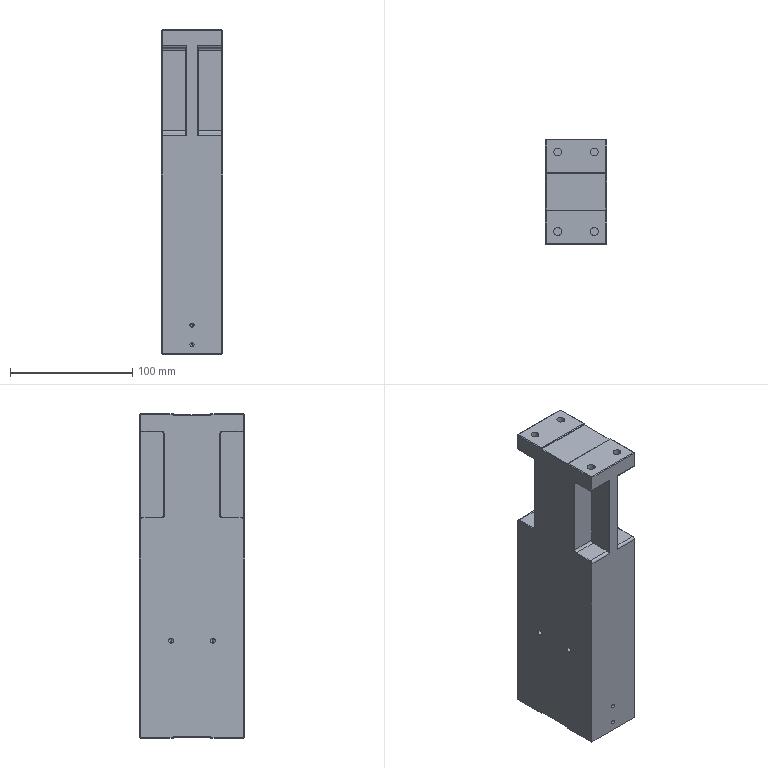Part | STEP file | 1 solid | 203 faces | box 50 x 86 x 266 mm | volume 1023683 mm3 | plane 102 | cylinder 57 | cone 44 | commonest cylinder face diameters 4 x16 5 x13 3.3 x12 4.2 x8 6.5 x8